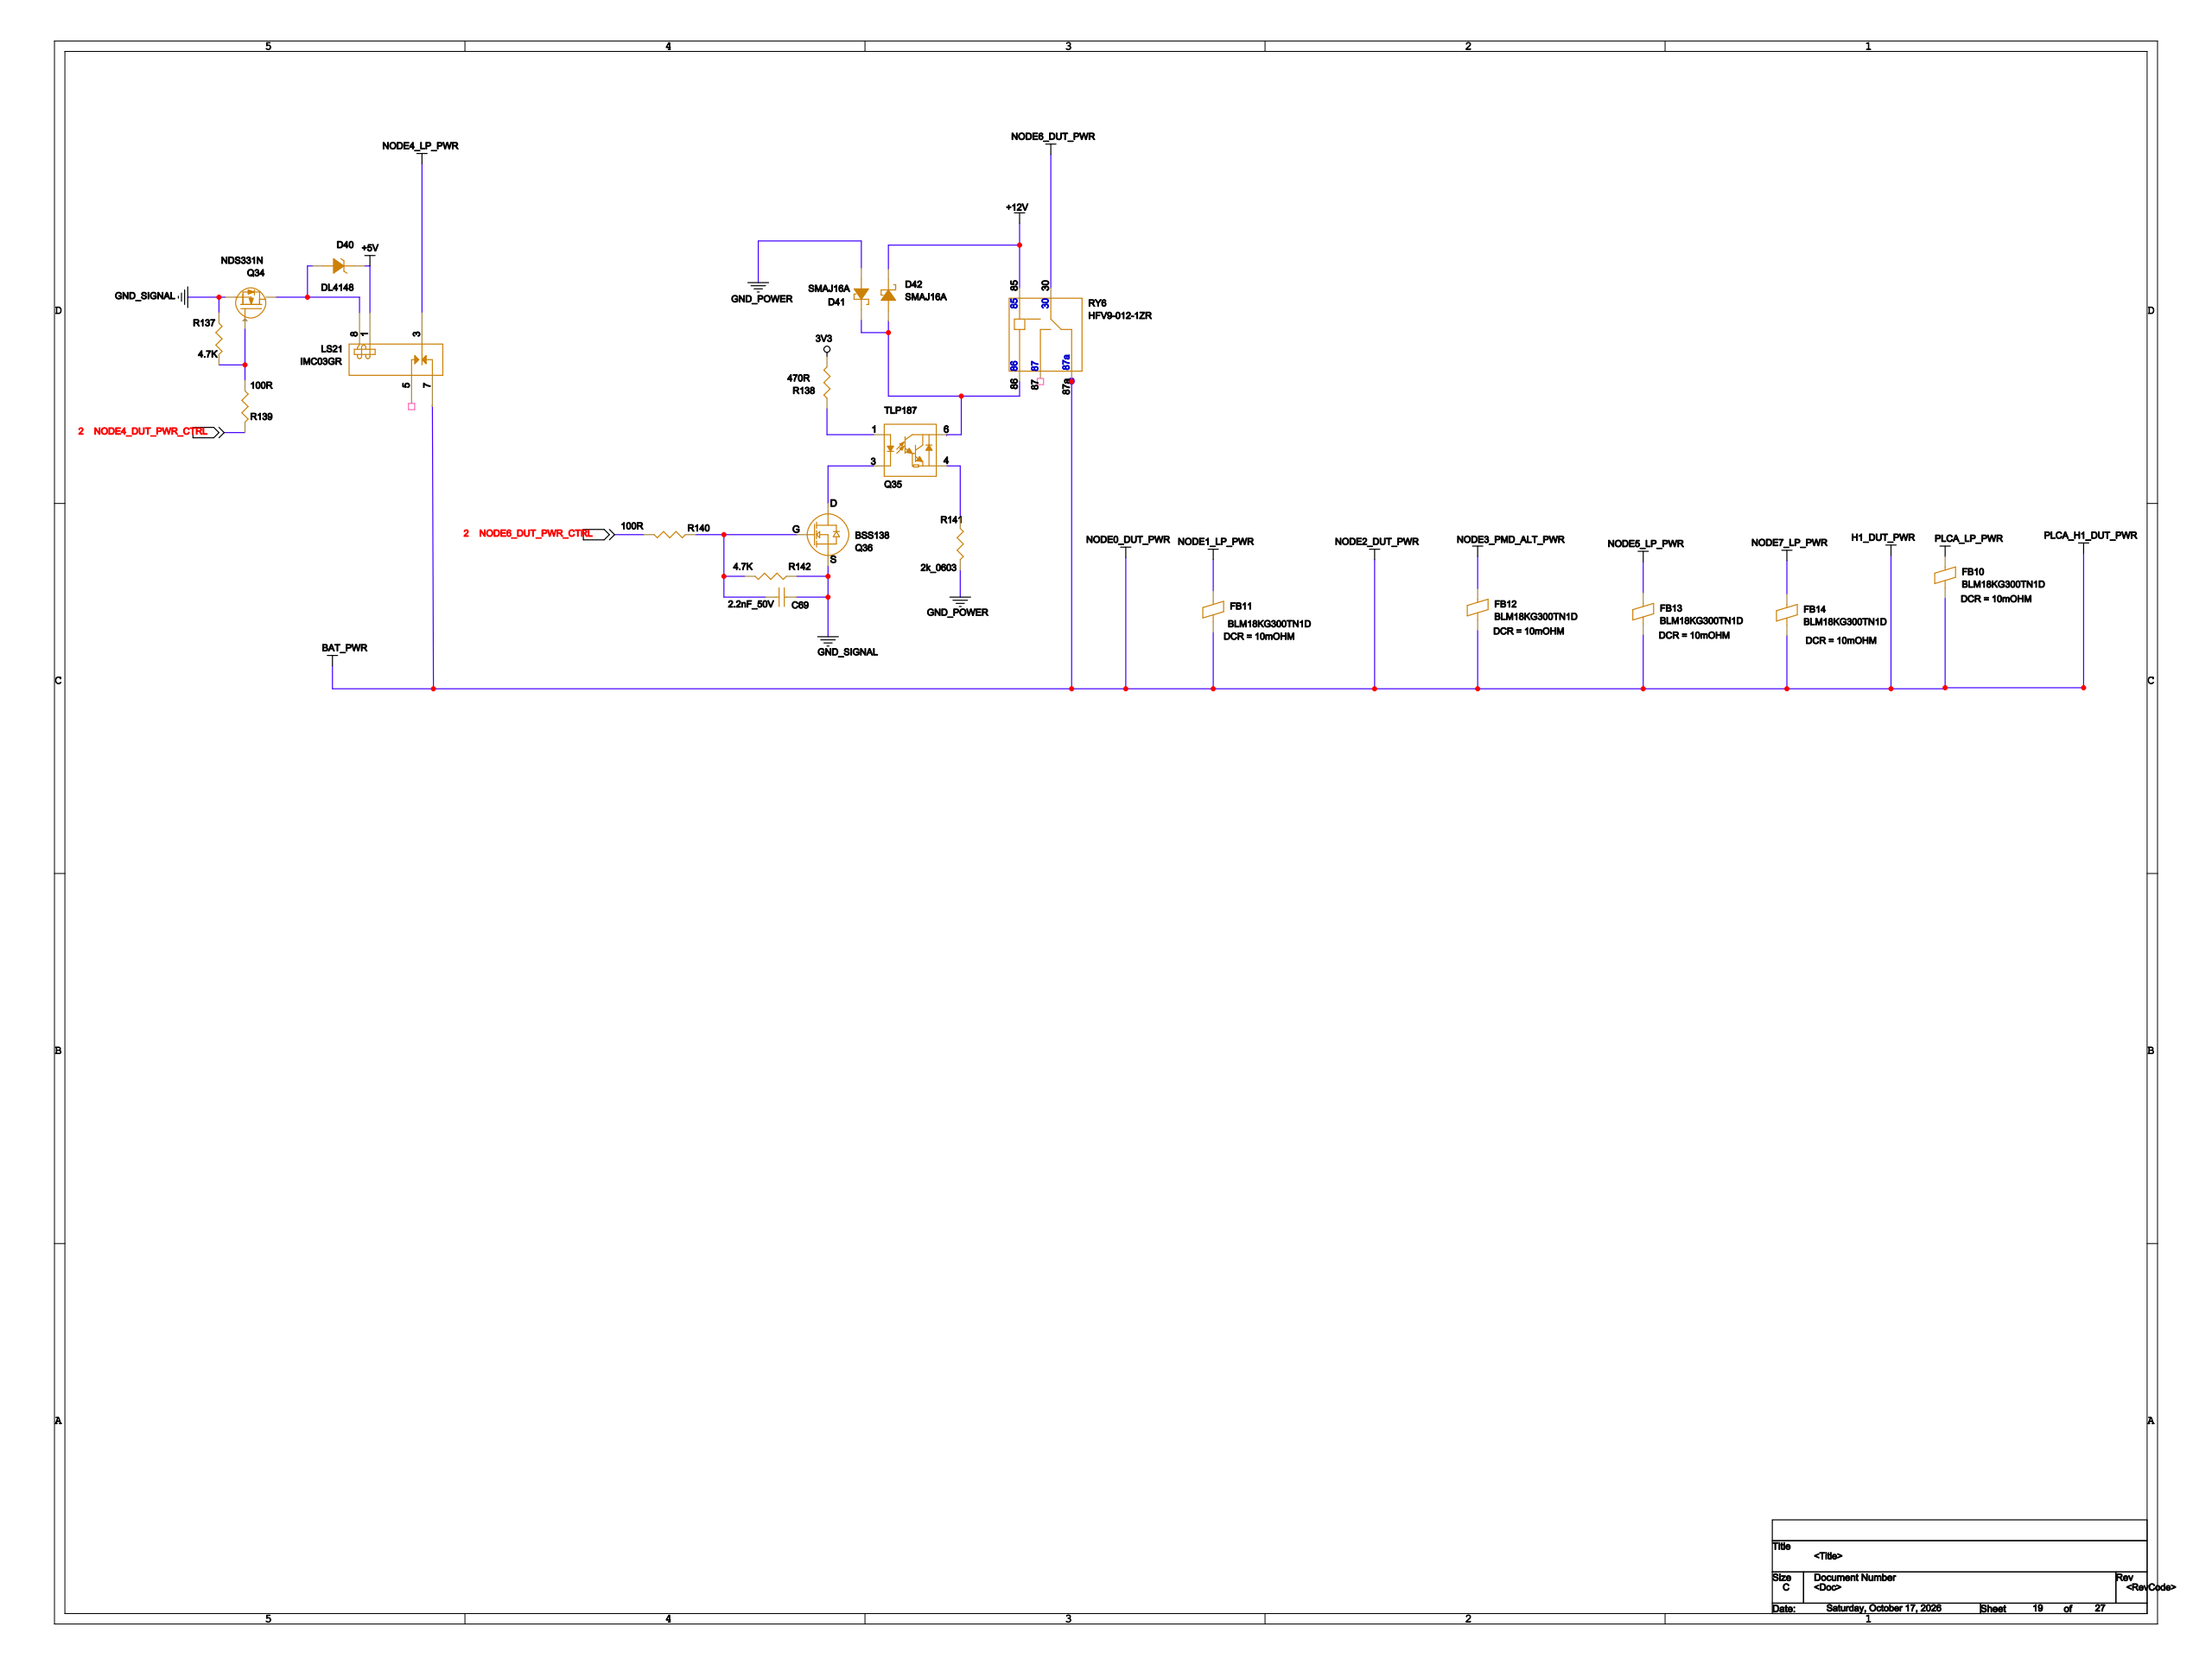Circuit board | Cadence Allegro | 477 parts | 327 nets | one sheet of the schematic
Parts on this sheet (reference | value | footprint):
C69 | 2.2nF_50V | 0603
D40 | DL4148 | MINIMELF
D41 | SMAJ16A | DO-214AC
D42 | SMAJ16A | DO-214AC
FB10 | BLM18KG300TN1D | 0603
FB11 | BLM18KG300TN1D | 0603
FB12 | BLM18KG300TN1D | 0603
FB13 | BLM18KG300TN1D | 0603
FB14 | BLM18KG300TN1D | 0603
LS21 | IMC03GR | IMC03GR
Q34 | NDS331N | SOT23-3
Q35 | TLP187 | TLP187
Q36 | BSS138 | 003_SOT23B
R137 | 4.7K | R0402
R138 | 470R | 0402
R139 | 100R | R0402
R140 | 100R | 0402
R141 | 2k_0603 | 0603
R142 | 4.7K | 0402
RY6 | HFV9-012-1ZR | HFV9-012-1ZR
Nets of these parts (net: part-pin ...):
N16913121: Q34-1 R137-2 R139-1
NODE4_DUT_PWR_CTRL: R139-2
BAT_GND: C69-1 D41-1 Q34-2 Q36-S R137-1 R141-2 R142-2
N16866088: C69-2 Q36-G R140-2 R142-1
3V3: R138-2
N16865970: Q35-1 R138-1
N16866016: Q35-4 R141-1
BAT_PWR: FB10-2 FB11-2 FB12-2 FB13-2 FB14-2 LS21-7 RY6-87A
+12V: D42-2 RY6-85
N16865894: D41-2 D42-1 Q35-6 RY6-86
NODE6_DUT_PWR: RY6-30
N16866012: Q35-3 Q36-D
+5V: D40-2 LS21-1
N16913077: D40-1 LS21-8 Q34-3
NODE5_LP_PWR: FB13-1
NODE7_LP_PWR: FB14-1
PLCA_LP_PWR: FB10-1
NODE1_LP_PWR: FB11-1
NODE3_PMD_ALT_PWR: FB12-1
NODE4_LP_PWR: LS21-3
NODE6_DUT_PWR_CTRL: R140-1